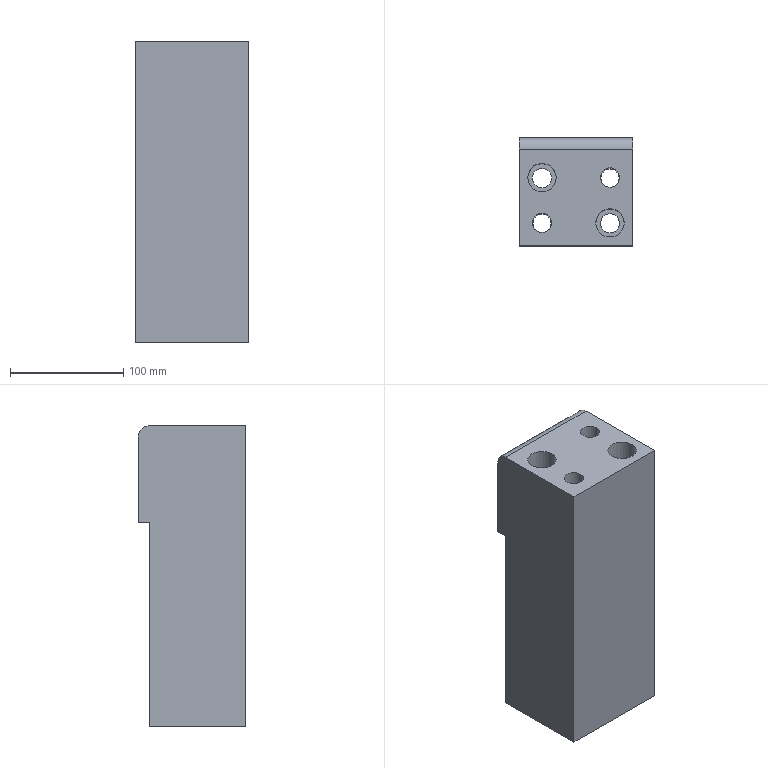Part | NX | features solid 2 | 1 solid | 21 faces | box 100 x 95 x 265 mm | volume 1972280 mm3 | plane 12 | cylinder 9 | commonest cylinder face diameters 17 x4 16 x2 25 x2 20 x1
STEP:
#1=CARTESIAN_POINT('',(347.5,-300.,85.));
#2=VERTEX_POINT('',#1);
#3=CARTESIAN_POINT('',(347.5,-215.,85.));
#4=VERTEX_POINT('',#3);
#5=CARTESIAN_POINT('',(347.5,-210.,85.));
#6=DIRECTION('',(0.,1.,0.));
#7=VECTOR('',#6,1000.);
#8=LINE('',#5,#7);
#9=EDGE_CURVE('',#2,#4,#8,.T.);
#10=ORIENTED_EDGE('',*,*,#9,.T.);
#11=CARTESIAN_POINT('',(347.5,-205.,75.));
#12=VERTEX_POINT('',#11);
#13=CARTESIAN_POINT('',(347.5,-215.,75.));
#14=DIRECTION('',(1.,0.,0.));
#15=DIRECTION('',(0.,0.,-1.));
#16=AXIS2_PLACEMENT_3D('',#13,#14,#15);
#17=CIRCLE('',#16,10.);
#18=EDGE_CURVE('',#4,#12,#17,.F.);
#19=ORIENTED_EDGE('',*,*,#18,.T.);
#20=CARTESIAN_POINT('',(347.5,-205.,0.));
#21=VERTEX_POINT('',#20);
#22=CARTESIAN_POINT('',(347.5,-205.,-75.));
#23=DIRECTION('',(0.,0.,1.));
#24=VECTOR('',#23,1000.);
#25=LINE('',#22,#24);
#26=EDGE_CURVE('',#21,#12,#25,.T.);
#27=ORIENTED_EDGE('',*,*,#26,.F.);
#28=CARTESIAN_POINT('',(347.5,-215.,0.));
#29=VERTEX_POINT('',#28);
#30=CARTESIAN_POINT('',(347.5,-210.,0.));
#31=DIRECTION('',(0.,1.,0.));
#32=VECTOR('',#31,1000.);
#33=LINE('',#30,#32);
#34=EDGE_CURVE('',#21,#29,#33,.F.);
#35=ORIENTED_EDGE('',*,*,#34,.T.);
#36=CARTESIAN_POINT('',(347.5,-215.,-180.));
#37=VERTEX_POINT('',#36);
#38=CARTESIAN_POINT('',(347.5,-215.,-75.));
#39=DIRECTION('',(0.,0.,1.));
#40=VECTOR('',#39,1000.);
#41=LINE('',#38,#40);
#42=EDGE_CURVE('',#29,#37,#41,.F.);
#43=ORIENTED_EDGE('',*,*,#42,.T.);
#44=CARTESIAN_POINT('',(347.5,-300.,-180.));
#45=VERTEX_POINT('',#44);
#46=CARTESIAN_POINT('',(347.5,-210.,-180.));
#47=DIRECTION('',(0.,-1.,0.));
#48=VECTOR('',#47,1000.);
#49=LINE('',#46,#48);
#50=EDGE_CURVE('',#37,#45,#49,.T.);
#51=ORIENTED_EDGE('',*,*,#50,.T.);
#52=CARTESIAN_POINT('',(347.5,-300.,-75.));
#53=DIRECTION('',(0.,0.,1.));
#54=VECTOR('',#53,1000.);
#55=LINE('',#52,#54);
#56=EDGE_CURVE('',#45,#2,#55,.T.);
#57=ORIENTED_EDGE('',*,*,#56,.T.);
#58=EDGE_LOOP('',(#10,#19,#27,#35,#43,#51,#57));
#59=FACE_BOUND('',#58,.T.);
#60=CARTESIAN_POINT('',(347.5,-210.,-75.));
#61=DIRECTION('',(1.,0.,0.));
#62=DIRECTION('',(0.,0.,-1.));
#63=AXIS2_PLACEMENT_3D('',#60,#61,#62);
#64=PLANE('',#63);
#65=ADVANCED_FACE('',(#59),#64,.F.);
#66=CARTESIAN_POINT('',(375.5,-280.,-180.));
#67=VERTEX_POINT('',#66);
#68=CARTESIAN_POINT('',(367.5,-280.,-180.));
#69=DIRECTION('',(0.,0.,1.));
#70=DIRECTION('',(1.,0.,0.));
#71=AXIS2_PLACEMENT_3D('',#68,#69,#70);
#72=CIRCLE('',#71,8.);
#73=EDGE_CURVE('',#67,#67,#72,.T.);
#74=ORIENTED_EDGE('',*,*,#73,.T.);
#75=EDGE_LOOP('',(#74));
#76=FACE_BOUND('',#75,.T.);
#77=CARTESIAN_POINT('',(435.5,-240.,-180.));
#78=VERTEX_POINT('',#77);
#79=CARTESIAN_POINT('',(427.5,-240.,-180.));
#80=DIRECTION('',(0.,0.,1.));
#81=DIRECTION('',(1.,0.,0.));
#82=AXIS2_PLACEMENT_3D('',#79,#80,#81);
#83=CIRCLE('',#82,8.);
#84=EDGE_CURVE('',#78,#78,#83,.T.);
#85=ORIENTED_EDGE('',*,*,#84,.T.);
#86=EDGE_LOOP('',(#85));
#87=FACE_BOUND('',#86,.T.);
#88=CARTESIAN_POINT('',(436.,-280.,-180.));
#89=VERTEX_POINT('',#88);
#90=CARTESIAN_POINT('',(427.5,-280.,-180.));
#91=DIRECTION('',(0.,0.,1.));
#92=DIRECTION('',(1.,0.,0.));
#93=AXIS2_PLACEMENT_3D('',#90,#91,#92);
#94=CIRCLE('',#93,8.5);
#95=EDGE_CURVE('',#89,#89,#94,.T.);
#96=ORIENTED_EDGE('',*,*,#95,.T.);
#97=EDGE_LOOP('',(#96));
#98=FACE_BOUND('',#97,.T.);
#99=CARTESIAN_POINT('',(376.,-240.,-180.));
#100=VERTEX_POINT('',#99);
#101=CARTESIAN_POINT('',(367.5,-240.,-180.));
#102=DIRECTION('',(0.,0.,1.));
#103=DIRECTION('',(1.,0.,0.));
#104=AXIS2_PLACEMENT_3D('',#101,#102,#103);
#105=CIRCLE('',#104,8.5);
#106=EDGE_CURVE('',#100,#100,#105,.T.);
#107=ORIENTED_EDGE('',*,*,#106,.T.);
#108=EDGE_LOOP('',(#107));
#109=FACE_BOUND('',#108,.T.);
#110=CARTESIAN_POINT('',(447.5,-215.,-180.));
#111=VERTEX_POINT('',#110);
#112=CARTESIAN_POINT('',(447.5,-215.,-180.));
#113=DIRECTION('',(-1.,0.,0.));
#114=VECTOR('',#113,1000.);
#115=LINE('',#112,#114);
#116=EDGE_CURVE('',#111,#37,#115,.T.);
#117=ORIENTED_EDGE('',*,*,#116,.F.);
#118=CARTESIAN_POINT('',(447.5,-300.,-180.));
#119=VERTEX_POINT('',#118);
#120=CARTESIAN_POINT('',(447.5,-210.,-180.));
#121=DIRECTION('',(0.,-1.,0.));
#122=VECTOR('',#121,1000.);
#123=LINE('',#120,#122);
#124=EDGE_CURVE('',#111,#119,#123,.T.);
#125=ORIENTED_EDGE('',*,*,#124,.T.);
#126=CARTESIAN_POINT('',(447.5,-300.,-180.));
#127=DIRECTION('',(-1.,0.,0.));
#128=VECTOR('',#127,1000.);
#129=LINE('',#126,#128);
#130=EDGE_CURVE('',#119,#45,#129,.T.);
#131=ORIENTED_EDGE('',*,*,#130,.T.);
#132=ORIENTED_EDGE('',*,*,#50,.F.);
#133=EDGE_LOOP('',(#117,#125,#131,#132));
#134=FACE_BOUND('',#133,.T.);
#135=CARTESIAN_POINT('',(447.5,-210.,-180.));
#136=DIRECTION('',(0.,0.,1.));
#137=DIRECTION('',(1.,0.,0.));
#138=AXIS2_PLACEMENT_3D('',#135,#136,#137);
#139=PLANE('',#138);
#140=ADVANCED_FACE('',(#76,#87,#98,#109,#134),#139,.F.);
#141=CARTESIAN_POINT('',(447.5,-205.,75.));
#142=VERTEX_POINT('',#141);
#143=CARTESIAN_POINT('',(447.5,-205.,0.));
#144=VERTEX_POINT('',#143);
#145=CARTESIAN_POINT('',(447.5,-205.,25.));
#146=DIRECTION('',(0.,0.,-1.));
#147=VECTOR('',#146,1000.);
#148=LINE('',#145,#147);
#149=EDGE_CURVE('',#142,#144,#148,.T.);
#150=ORIENTED_EDGE('',*,*,#149,.F.);
#151=CARTESIAN_POINT('',(447.5,-215.,85.));
#152=VERTEX_POINT('',#151);
#153=CARTESIAN_POINT('',(447.5,-215.,75.));
#154=DIRECTION('',(-1.,0.,0.));
#155=DIRECTION('',(0.,0.,1.));
#156=AXIS2_PLACEMENT_3D('',#153,#154,#155);
#157=CIRCLE('',#156,10.);
#158=EDGE_CURVE('',#142,#152,#157,.F.);
#159=ORIENTED_EDGE('',*,*,#158,.T.);
#160=CARTESIAN_POINT('',(447.5,-300.,85.));
#161=VERTEX_POINT('',#160);
#162=CARTESIAN_POINT('',(447.5,-210.,85.));
#163=DIRECTION('',(0.,-1.,0.));
#164=VECTOR('',#163,1000.);
#165=LINE('',#162,#164);
#166=EDGE_CURVE('',#152,#161,#165,.T.);
#167=ORIENTED_EDGE('',*,*,#166,.T.);
#168=CARTESIAN_POINT('',(447.5,-300.,25.));
#169=DIRECTION('',(0.,0.,-1.));
#170=VECTOR('',#169,1000.);
#171=LINE('',#168,#170);
#172=EDGE_CURVE('',#161,#119,#171,.T.);
#173=ORIENTED_EDGE('',*,*,#172,.T.);
#174=ORIENTED_EDGE('',*,*,#124,.F.);
#175=CARTESIAN_POINT('',(447.5,-215.,0.));
#176=VERTEX_POINT('',#175);
#177=CARTESIAN_POINT('',(447.5,-215.,-75.));
#178=DIRECTION('',(0.,0.,1.));
#179=VECTOR('',#178,1000.);
#180=LINE('',#177,#179);
#181=EDGE_CURVE('',#176,#111,#180,.F.);
#182=ORIENTED_EDGE('',*,*,#181,.F.);
#183=CARTESIAN_POINT('',(447.5,-210.,0.));
#184=DIRECTION('',(0.,1.,0.));
#185=VECTOR('',#184,1000.);
#186=LINE('',#183,#185);
#187=EDGE_CURVE('',#144,#176,#186,.F.);
#188=ORIENTED_EDGE('',*,*,#187,.F.);
#189=EDGE_LOOP('',(#150,#159,#167,#173,#174,#182,#188));
#190=FACE_BOUND('',#189,.T.);
#191=CARTESIAN_POINT('',(447.5,-210.,25.));
#192=DIRECTION('',(-1.,0.,0.));
#193=DIRECTION('',(0.,0.,1.));
#194=AXIS2_PLACEMENT_3D('',#191,#192,#193);
#195=PLANE('',#194);
#196=ADVANCED_FACE('',(#190),#195,.F.);
#197=ORIENTED_EDGE('',*,*,#26,.T.);
#198=CARTESIAN_POINT('',(447.5,-205.,75.));
#199=DIRECTION('',(1.,0.,0.));
#200=VECTOR('',#199,1000.);
#201=LINE('',#198,#200);
#202=EDGE_CURVE('',#12,#142,#201,.T.);
#203=ORIENTED_EDGE('',*,*,#202,.T.);
#204=ORIENTED_EDGE('',*,*,#149,.T.);
#205=CARTESIAN_POINT('',(447.5,-205.,0.));
#206=DIRECTION('',(1.,0.,0.));
#207=VECTOR('',#206,1000.);
#208=LINE('',#205,#207);
#209=EDGE_CURVE('',#144,#21,#208,.F.);
#210=ORIENTED_EDGE('',*,*,#209,.T.);
#211=EDGE_LOOP('',(#197,#203,#204,#210));
#212=FACE_BOUND('',#211,.T.);
#213=CARTESIAN_POINT('',(447.5,-205.,25.));
#214=DIRECTION('',(0.,1.,0.));
#215=DIRECTION('',(-1.,0.,0.));
#216=AXIS2_PLACEMENT_3D('',#213,#214,#215);
#217=PLANE('',#216);
#218=ADVANCED_FACE('',(#212),#217,.T.);
#219=CARTESIAN_POINT('',(359.,-280.,85.));
#220=VERTEX_POINT('',#219);
#221=CARTESIAN_POINT('',(367.5,-280.,85.));
#222=DIRECTION('',(0.,0.,-1.));
#223=DIRECTION('',(-1.,0.,0.));
#224=AXIS2_PLACEMENT_3D('',#221,#222,#223);
#225=CIRCLE('',#224,8.5);
#226=EDGE_CURVE('',#220,#220,#225,.T.);
#227=ORIENTED_EDGE('',*,*,#226,.T.);
#228=EDGE_LOOP('',(#227));
#229=FACE_BOUND('',#228,.T.);
#230=CARTESIAN_POINT('',(419.,-240.,85.));
#231=VERTEX_POINT('',#230);
#232=CARTESIAN_POINT('',(427.5,-240.,85.));
#233=DIRECTION('',(0.,0.,-1.));
#234=DIRECTION('',(-1.,0.,0.));
#235=AXIS2_PLACEMENT_3D('',#232,#233,#234);
#236=CIRCLE('',#235,8.5);
#237=EDGE_CURVE('',#231,#231,#236,.T.);
#238=ORIENTED_EDGE('',*,*,#237,.T.);
#239=EDGE_LOOP('',(#238));
#240=FACE_BOUND('',#239,.T.);
#241=CARTESIAN_POINT('',(415.,-280.,85.));
#242=VERTEX_POINT('',#241);
#243=CARTESIAN_POINT('',(427.5,-280.,85.));
#244=DIRECTION('',(0.,0.,-1.));
#245=DIRECTION('',(-1.,0.,0.));
#246=AXIS2_PLACEMENT_3D('',#243,#244,#245);
#247=CIRCLE('',#246,12.5);
#248=EDGE_CURVE('',#242,#242,#247,.T.);
#249=ORIENTED_EDGE('',*,*,#248,.T.);
#250=EDGE_LOOP('',(#249));
#251=FACE_BOUND('',#250,.T.);
#252=CARTESIAN_POINT('',(355.,-240.,85.));
#253=VERTEX_POINT('',#252);
#254=CARTESIAN_POINT('',(367.5,-240.,85.));
#255=DIRECTION('',(0.,0.,-1.));
#256=DIRECTION('',(-1.,0.,0.));
#257=AXIS2_PLACEMENT_3D('',#254,#255,#256);
#258=CIRCLE('',#257,12.5);
#259=EDGE_CURVE('',#253,#253,#258,.T.);
#260=ORIENTED_EDGE('',*,*,#259,.T.);
#261=EDGE_LOOP('',(#260));
#262=FACE_BOUND('',#261,.T.);
#263=ORIENTED_EDGE('',*,*,#166,.F.);
#264=CARTESIAN_POINT('',(347.5,-215.,85.));
#265=DIRECTION('',(1.,0.,0.));
#266=VECTOR('',#265,1000.);
#267=LINE('',#264,#266);
#268=EDGE_CURVE('',#152,#4,#267,.F.);
#269=ORIENTED_EDGE('',*,*,#268,.T.);
#270=ORIENTED_EDGE('',*,*,#9,.F.);
#271=CARTESIAN_POINT('',(447.5,-300.,85.));
#272=DIRECTION('',(-1.,0.,0.));
#273=VECTOR('',#272,1000.);
#274=LINE('',#271,#273);
#275=EDGE_CURVE('',#161,#2,#274,.T.);
#276=ORIENTED_EDGE('',*,*,#275,.F.);
#277=EDGE_LOOP('',(#263,#269,#270,#276));
#278=FACE_BOUND('',#277,.T.);
#279=CARTESIAN_POINT('',(372.5,-210.,85.));
#280=DIRECTION('',(0.,0.,-1.));
#281=DIRECTION('',(-1.,0.,0.));
#282=AXIS2_PLACEMENT_3D('',#279,#280,#281);
#283=PLANE('',#282);
#284=ADVANCED_FACE('',(#229,#240,#251,#262,#278),#283,.F.);
#285=ORIENTED_EDGE('',*,*,#172,.F.);
#286=ORIENTED_EDGE('',*,*,#275,.T.);
#287=ORIENTED_EDGE('',*,*,#56,.F.);
#288=ORIENTED_EDGE('',*,*,#130,.F.);
#289=EDGE_LOOP('',(#285,#286,#287,#288));
#290=FACE_BOUND('',#289,.T.);
#291=CARTESIAN_POINT('',(447.5,-300.,25.));
#292=DIRECTION('',(0.,1.,0.));
#293=DIRECTION('',(-1.,0.,0.));
#294=AXIS2_PLACEMENT_3D('',#291,#292,#293);
#295=PLANE('',#294);
#296=ADVANCED_FACE('',(#290),#295,.F.);
#297=ORIENTED_EDGE('',*,*,#116,.T.);
#298=ORIENTED_EDGE('',*,*,#42,.F.);
#299=CARTESIAN_POINT('',(347.5,-215.,0.));
#300=DIRECTION('',(-1.,0.,0.));
#301=VECTOR('',#300,1000.);
#302=LINE('',#299,#301);
#303=EDGE_CURVE('',#29,#176,#302,.F.);
#304=ORIENTED_EDGE('',*,*,#303,.T.);
#305=ORIENTED_EDGE('',*,*,#181,.T.);
#306=EDGE_LOOP('',(#297,#298,#304,#305));
#307=FACE_BOUND('',#306,.T.);
#308=CARTESIAN_POINT('',(347.5,-215.,-75.));
#309=DIRECTION('',(0.,1.,0.));
#310=DIRECTION('',(0.,0.,1.));
#311=AXIS2_PLACEMENT_3D('',#308,#309,#310);
#312=PLANE('',#311);
#313=ADVANCED_FACE('',(#307),#312,.T.);
#314=ORIENTED_EDGE('',*,*,#187,.T.);
#315=ORIENTED_EDGE('',*,*,#303,.F.);
#316=ORIENTED_EDGE('',*,*,#34,.F.);
#317=ORIENTED_EDGE('',*,*,#209,.F.);
#318=EDGE_LOOP('',(#314,#315,#316,#317));
#319=FACE_BOUND('',#318,.T.);
#320=CARTESIAN_POINT('',(347.5,-210.,0.));
#321=DIRECTION('',(0.,0.,1.));
#322=DIRECTION('',(1.,0.,0.));
#323=AXIS2_PLACEMENT_3D('',#320,#321,#322);
#324=PLANE('',#323);
#325=ADVANCED_FACE('',(#319),#324,.F.);
#326=ORIENTED_EDGE('',*,*,#18,.F.);
#327=ORIENTED_EDGE('',*,*,#268,.F.);
#328=ORIENTED_EDGE('',*,*,#158,.F.);
#329=ORIENTED_EDGE('',*,*,#202,.F.);
#330=EDGE_LOOP('',(#326,#327,#328,#329));
#331=FACE_BOUND('',#330,.T.);
#332=CARTESIAN_POINT('',(447.5,-215.,75.));
#333=DIRECTION('',(-1.,0.,0.));
#334=DIRECTION('',(0.,0.,1.));
#335=AXIS2_PLACEMENT_3D('',#332,#333,#334);
#336=CYLINDRICAL_SURFACE('',#335,10.);
#337=ADVANCED_FACE('',(#331),#336,.T.);
#338=CARTESIAN_POINT('',(359.,-240.,-150.));
#339=VERTEX_POINT('',#338);
#340=CARTESIAN_POINT('',(367.5,-240.,-150.));
#341=DIRECTION('',(0.,0.,-1.));
#342=DIRECTION('',(-1.,0.,0.));
#343=AXIS2_PLACEMENT_3D('',#340,#341,#342);
#344=CIRCLE('',#343,8.5);
#345=EDGE_CURVE('',#339,#339,#344,.F.);
#346=ORIENTED_EDGE('',*,*,#345,.T.);
#347=EDGE_LOOP('',(#346));
#348=FACE_BOUND('',#347,.T.);
#349=ORIENTED_EDGE('',*,*,#106,.F.);
#350=EDGE_LOOP('',(#349));
#351=FACE_BOUND('',#350,.T.);
#352=CARTESIAN_POINT('',(367.5,-240.,-210.));
#353=DIRECTION('',(0.,0.,1.));
#354=DIRECTION('',(1.,0.,0.));
#355=AXIS2_PLACEMENT_3D('',#352,#353,#354);
#356=CYLINDRICAL_SURFACE('',#355,8.5);
#357=ADVANCED_FACE('',(#348,#351),#356,.F.);
#358=CARTESIAN_POINT('',(380.,-240.,-150.));
#359=VERTEX_POINT('',#358);
#360=CARTESIAN_POINT('',(367.5,-240.,-150.));
#361=DIRECTION('',(0.,0.,1.));
#362=DIRECTION('',(1.,0.,0.));
#363=AXIS2_PLACEMENT_3D('',#360,#361,#362);
#364=CIRCLE('',#363,12.5);
#365=EDGE_CURVE('',#359,#359,#364,.T.);
#366=ORIENTED_EDGE('',*,*,#365,.F.);
#367=EDGE_LOOP('',(#366));
#368=FACE_BOUND('',#367,.T.);
#369=ORIENTED_EDGE('',*,*,#259,.F.);
#370=EDGE_LOOP('',(#369));
#371=FACE_BOUND('',#370,.T.);
#372=CARTESIAN_POINT('',(367.5,-240.,-150.));
#373=DIRECTION('',(0.,0.,1.));
#374=DIRECTION('',(1.,0.,0.));
#375=AXIS2_PLACEMENT_3D('',#372,#373,#374);
#376=CYLINDRICAL_SURFACE('',#375,12.5);
#377=ADVANCED_FACE('',(#368,#371),#376,.F.);
#378=ORIENTED_EDGE('',*,*,#345,.F.);
#379=EDGE_LOOP('',(#378));
#380=FACE_BOUND('',#379,.T.);
#381=ORIENTED_EDGE('',*,*,#365,.T.);
#382=EDGE_LOOP('',(#381));
#383=FACE_BOUND('',#382,.T.);
#384=CARTESIAN_POINT('',(367.5,-240.,-150.));
#385=DIRECTION('',(0.,0.,-1.));
#386=DIRECTION('',(-1.,0.,0.));
#387=AXIS2_PLACEMENT_3D('',#384,#385,#386);
#388=PLANE('',#387);
#389=ADVANCED_FACE('',(#380,#383),#388,.F.);
#390=CARTESIAN_POINT('',(419.,-280.,-150.));
#391=VERTEX_POINT('',#390);
#392=CARTESIAN_POINT('',(427.5,-280.,-150.));
#393=DIRECTION('',(0.,0.,-1.));
#394=DIRECTION('',(-1.,0.,0.));
#395=AXIS2_PLACEMENT_3D('',#392,#393,#394);
#396=CIRCLE('',#395,8.5);
#397=EDGE_CURVE('',#391,#391,#396,.F.);
#398=ORIENTED_EDGE('',*,*,#397,.T.);
#399=EDGE_LOOP('',(#398));
#400=FACE_BOUND('',#399,.T.);
#401=ORIENTED_EDGE('',*,*,#95,.F.);
#402=EDGE_LOOP('',(#401));
#403=FACE_BOUND('',#402,.T.);
#404=CARTESIAN_POINT('',(427.5,-280.,-210.));
#405=DIRECTION('',(0.,0.,1.));
#406=DIRECTION('',(1.,0.,0.));
#407=AXIS2_PLACEMENT_3D('',#404,#405,#406);
#408=CYLINDRICAL_SURFACE('',#407,8.5);
#409=ADVANCED_FACE('',(#400,#403),#408,.F.);
#410=CARTESIAN_POINT('',(440.,-280.,-150.));
#411=VERTEX_POINT('',#410);
#412=CARTESIAN_POINT('',(427.5,-280.,-150.));
#413=DIRECTION('',(0.,0.,1.));
#414=DIRECTION('',(1.,0.,0.));
#415=AXIS2_PLACEMENT_3D('',#412,#413,#414);
#416=CIRCLE('',#415,12.5);
#417=EDGE_CURVE('',#411,#411,#416,.T.);
#418=ORIENTED_EDGE('',*,*,#417,.F.);
#419=EDGE_LOOP('',(#418));
#420=FACE_BOUND('',#419,.T.);
#421=ORIENTED_EDGE('',*,*,#248,.F.);
#422=EDGE_LOOP('',(#421));
#423=FACE_BOUND('',#422,.T.);
#424=CARTESIAN_POINT('',(427.5,-280.,-150.));
#425=DIRECTION('',(0.,0.,1.));
#426=DIRECTION('',(1.,0.,0.));
#427=AXIS2_PLACEMENT_3D('',#424,#425,#426);
#428=CYLINDRICAL_SURFACE('',#427,12.5);
#429=ADVANCED_FACE('',(#420,#423),#428,.F.);
#430=ORIENTED_EDGE('',*,*,#397,.F.);
#431=EDGE_LOOP('',(#430));
#432=FACE_BOUND('',#431,.T.);
#433=ORIENTED_EDGE('',*,*,#417,.T.);
#434=EDGE_LOOP('',(#433));
#435=FACE_BOUND('',#434,.T.);
#436=CARTESIAN_POINT('',(427.5,-280.,-150.));
#437=DIRECTION('',(0.,0.,-1.));
#438=DIRECTION('',(-1.,0.,0.));
#439=AXIS2_PLACEMENT_3D('',#436,#437,#438);
#440=PLANE('',#439);
#441=ADVANCED_FACE('',(#432,#435),#440,.F.);
#442=CARTESIAN_POINT('',(419.5,-240.,-150.));
#443=VERTEX_POINT('',#442);
#444=CARTESIAN_POINT('',(427.5,-240.,-150.));
#445=DIRECTION('',(0.,0.,-1.));
#446=DIRECTION('',(-1.,0.,0.));
#447=AXIS2_PLACEMENT_3D('',#444,#445,#446);
#448=CIRCLE('',#447,8.);
#449=EDGE_CURVE('',#443,#443,#448,.F.);
#450=ORIENTED_EDGE('',*,*,#449,.T.);
#451=EDGE_LOOP('',(#450));
#452=FACE_BOUND('',#451,.T.);
#453=ORIENTED_EDGE('',*,*,#84,.F.);
#454=EDGE_LOOP('',(#453));
#455=FACE_BOUND('',#454,.T.);
#456=CARTESIAN_POINT('',(427.5,-240.,-210.));
#457=DIRECTION('',(0.,0.,1.));
#458=DIRECTION('',(1.,0.,0.));
#459=AXIS2_PLACEMENT_3D('',#456,#457,#458);
#460=CYLINDRICAL_SURFACE('',#459,8.);
#461=ADVANCED_FACE('',(#452,#455),#460,.F.);
#462=CARTESIAN_POINT('',(436.,-240.,-150.));
#463=VERTEX_POINT('',#462);
#464=CARTESIAN_POINT('',(427.5,-240.,-150.));
#465=DIRECTION('',(0.,0.,1.));
#466=DIRECTION('',(1.,0.,0.));
#467=AXIS2_PLACEMENT_3D('',#464,#465,#466);
#468=CIRCLE('',#467,8.5);
#469=EDGE_CURVE('',#463,#463,#468,.T.);
#470=ORIENTED_EDGE('',*,*,#469,.F.);
#471=EDGE_LOOP('',(#470));
#472=FACE_BOUND('',#471,.T.);
#473=ORIENTED_EDGE('',*,*,#237,.F.);
#474=EDGE_LOOP('',(#473));
#475=FACE_BOUND('',#474,.T.);
#476=CARTESIAN_POINT('',(427.5,-240.,-150.));
#477=DIRECTION('',(0.,0.,1.));
#478=DIRECTION('',(1.,0.,0.));
#479=AXIS2_PLACEMENT_3D('',#476,#477,#478);
#480=CYLINDRICAL_SURFACE('',#479,8.5);
#481=ADVANCED_FACE('',(#472,#475),#480,.F.);
#482=ORIENTED_EDGE('',*,*,#449,.F.);
#483=EDGE_LOOP('',(#482));
#484=FACE_BOUND('',#483,.T.);
#485=ORIENTED_EDGE('',*,*,#469,.T.);
#486=EDGE_LOOP('',(#485));
#487=FACE_BOUND('',#486,.T.);
#488=CARTESIAN_POINT('',(427.5,-240.,-150.));
#489=DIRECTION('',(0.,0.,-1.));
#490=DIRECTION('',(-1.,0.,0.));
#491=AXIS2_PLACEMENT_3D('',#488,#489,#490);
#492=PLANE('',#491);
#493=ADVANCED_FACE('',(#484,#487),#492,.F.);
#494=CARTESIAN_POINT('',(359.5,-280.,-150.));
#495=VERTEX_POINT('',#494);
#496=CARTESIAN_POINT('',(367.5,-280.,-150.));
#497=DIRECTION('',(0.,0.,-1.));
#498=DIRECTION('',(-1.,0.,0.));
#499=AXIS2_PLACEMENT_3D('',#496,#497,#498);
#500=CIRCLE('',#499,8.);
#501=EDGE_CURVE('',#495,#495,#500,.F.);
#502=ORIENTED_EDGE('',*,*,#501,.T.);
#503=EDGE_LOOP('',(#502));
#504=FACE_BOUND('',#503,.T.);
#505=ORIENTED_EDGE('',*,*,#73,.F.);
#506=EDGE_LOOP('',(#505));
#507=FACE_BOUND('',#506,.T.);
#508=CARTESIAN_POINT('',(367.5,-280.,-210.));
#509=DIRECTION('',(0.,0.,1.));
#510=DIRECTION('',(1.,0.,0.));
#511=AXIS2_PLACEMENT_3D('',#508,#509,#510);
#512=CYLINDRICAL_SURFACE('',#511,8.);
#513=ADVANCED_FACE('',(#504,#507),#512,.F.);
#514=CARTESIAN_POINT('',(376.,-280.,-150.));
#515=VERTEX_POINT('',#514);
#516=CARTESIAN_POINT('',(367.5,-280.,-150.));
#517=DIRECTION('',(0.,0.,1.));
#518=DIRECTION('',(1.,0.,0.));
#519=AXIS2_PLACEMENT_3D('',#516,#517,#518);
#520=CIRCLE('',#519,8.5);
#521=EDGE_CURVE('',#515,#515,#520,.T.);
#522=ORIENTED_EDGE('',*,*,#521,.F.);
#523=EDGE_LOOP('',(#522));
#524=FACE_BOUND('',#523,.T.);
#525=ORIENTED_EDGE('',*,*,#226,.F.);
#526=EDGE_LOOP('',(#525));
#527=FACE_BOUND('',#526,.T.);
#528=CARTESIAN_POINT('',(367.5,-280.,-150.));
#529=DIRECTION('',(0.,0.,1.));
#530=DIRECTION('',(1.,0.,0.));
#531=AXIS2_PLACEMENT_3D('',#528,#529,#530);
#532=CYLINDRICAL_SURFACE('',#531,8.5);
#533=ADVANCED_FACE('',(#524,#527),#532,.F.);
#534=ORIENTED_EDGE('',*,*,#501,.F.);
#535=EDGE_LOOP('',(#534));
#536=FACE_BOUND('',#535,.T.);
#537=ORIENTED_EDGE('',*,*,#521,.T.);
#538=EDGE_LOOP('',(#537));
#539=FACE_BOUND('',#538,.T.);
#540=CARTESIAN_POINT('',(367.5,-280.,-150.));
#541=DIRECTION('',(0.,0.,-1.));
#542=DIRECTION('',(-1.,0.,0.));
#543=AXIS2_PLACEMENT_3D('',#540,#541,#542);
#544=PLANE('',#543);
#545=ADVANCED_FACE('',(#536,#539),#544,.F.);
#546=CLOSED_SHELL('',(#65,#140,#196,#218,#284,#296,#313,#325,#337,#357,#377,#389,#409,#429,#441,#461,#481,#493,#513,#533,#545));
#547=MANIFOLD_SOLID_BREP('',#546);
#548=(LENGTH_UNIT()NAMED_UNIT(*)SI_UNIT(.MILLI.,.METRE.));
#549=UNCERTAINTY_MEASURE_WITH_UNIT(LENGTH_MEASURE(0.00001),#548,'','');
#550=(NAMED_UNIT(*)PLANE_ANGLE_UNIT()SI_UNIT($,.RADIAN.));
#551=(NAMED_UNIT(*)SI_UNIT($,.STERADIAN.)SOLID_ANGLE_UNIT());
#552=(GEOMETRIC_REPRESENTATION_CONTEXT(3)GLOBAL_UNCERTAINTY_ASSIGNED_CONTEXT((#549))GLOBAL_UNIT_ASSIGNED_CONTEXT((#548,#550,#551))REPRESENTATION_CONTEXT('',''));
#553=ADVANCED_BREP_SHAPE_REPRESENTATION('',(#547),#552);